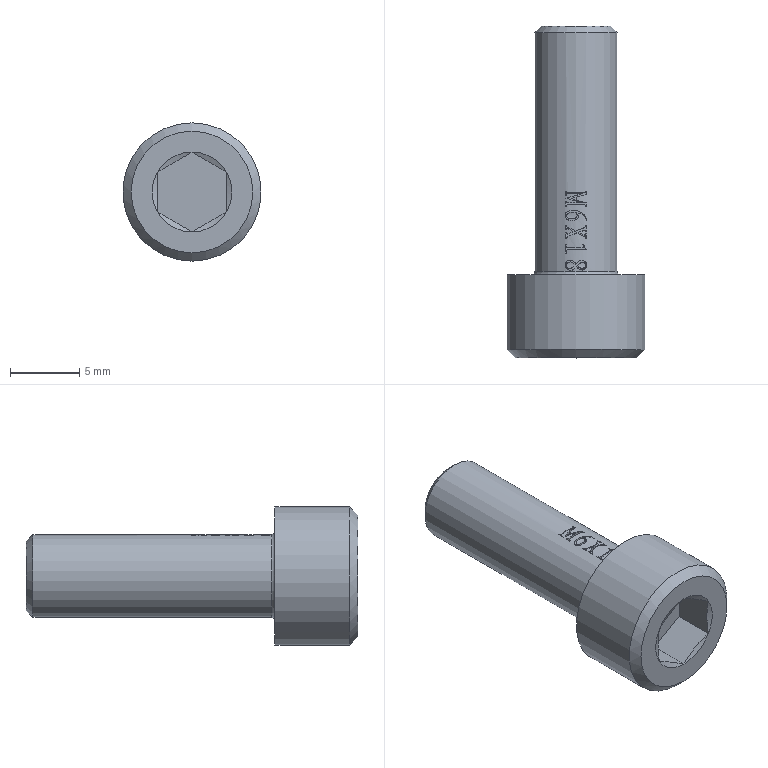Part | STEP file | solid 103 | 1 solid | 105 faces | box 10 x 24 x 10 mm | volume 907.17 mm3 | plane 53 | other 35 | cylinder 8 | sphere 6 | cone 2 | torus 1 | commonest cylinder face diameters 6 x7 10 x1